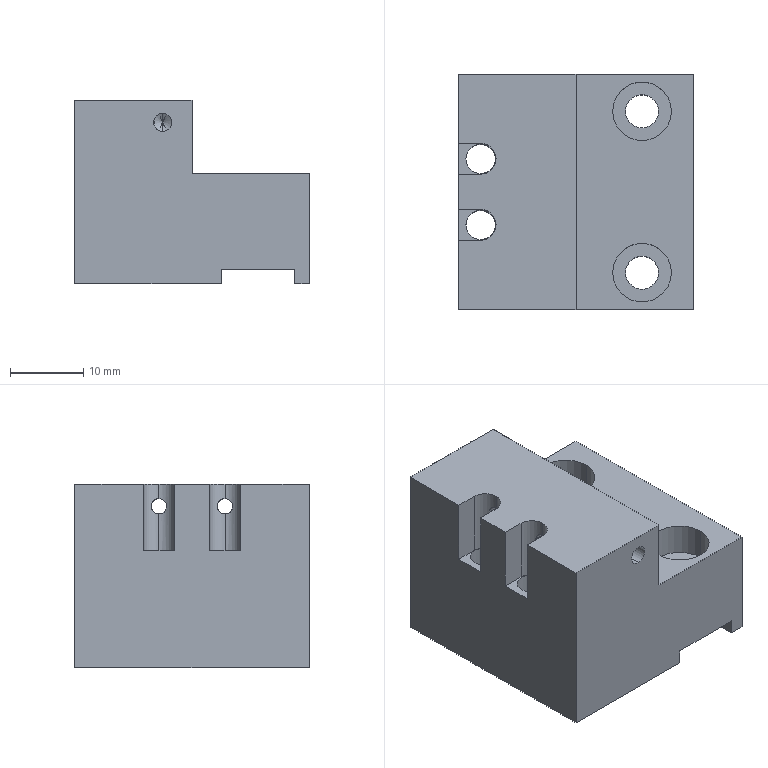Part | STEP file | B03 | 1 solid | 52 faces | box 32 x 32 x 25 mm | volume 18185 mm3 | cylinder 28 | plane 20 | cone 4 | commonest cylinder face diameters 2.1 x8 2.5 x4 4 x4 4.2 x4 4.5 x4 8 x4